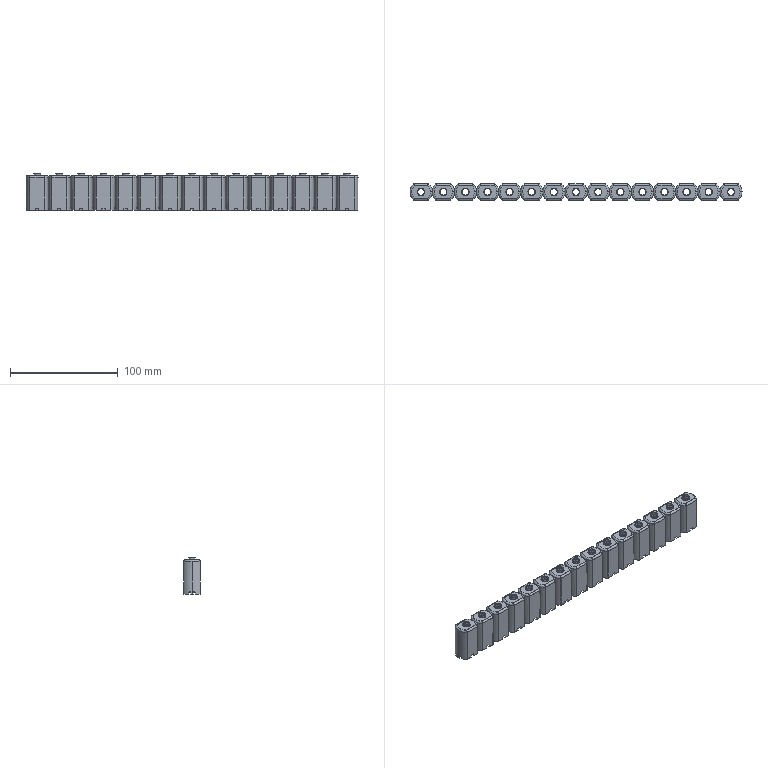Part | STEP file | shell block | 15 solids | 765 faces | box 307.5 x 15.4 x 34 mm | volume 6550 mm3 | plane 345 | cylinder 270 | torus 150 | commonest cylinder face diameters 1.608 x60 20.1 x45 20.5 x45 3 x30 3.4 x30 6 x30